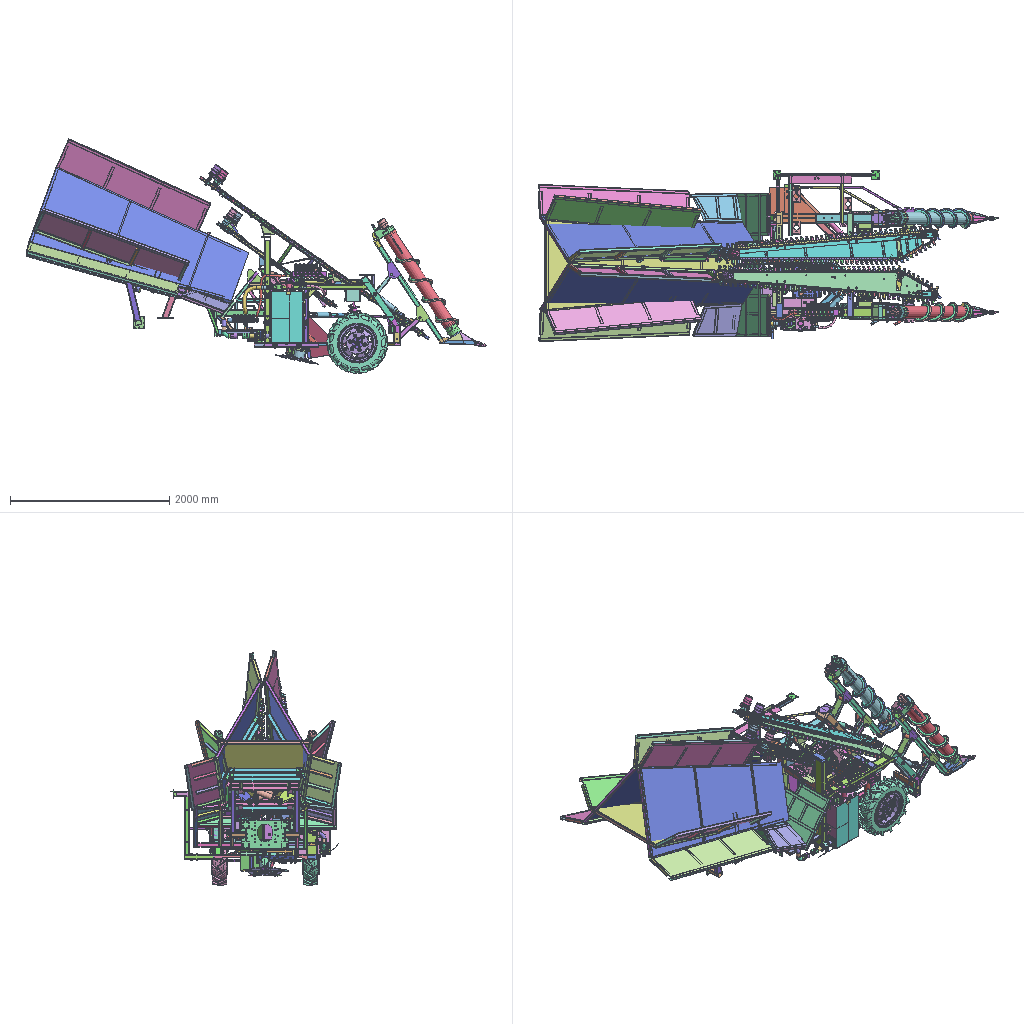Assembly | STEP file | 173 different items | 615 placed | box 5779 x 2151 x 2951 mm
Parts list (item | name | quantity | parent item | size | volume):
1 | 1 exported frame why_stp | x1 | in sugarcane cutter-windrower module--20251214 | 80 x 1320 x 1285 mm | 10409301 mm3
2 | floating channel bottom plate--2025.12.03 | x1 | in floating channel--20251204 | 466.015 x 268.5 x 616.159 mm | 643321 mm3
3 | floating channel right front section | x1 | in floating channel--20251204 | 394.503 x 166.964 x 591.584 mm | 406716 mm3
4 | floating channel left front section | x1 | in floating channel--20251204 | 372.026 x 168.494 x 590.246 mm | 526748 mm3
5 | floating channel side plate | x1 | in floating channel--20251204 | 471.639 x 3 x 716.945 mm | 405193 mm3
6 | floating channel side plate 02 | x1 | in floating channel--20251204 | 470.946 x 3 x 716.27 mm | 404515 mm3
7 | support fixing frame | x1 | in floating channel fixing frame_MODEL | 66.075 x 284.5 x 50.67 mm | 158932 mm3
8 | vertical fixing frame | x1 | in floating channel fixing frame_MODEL | 87.186 x 40 x 183.865 mm | 87563 mm3
9 | diagonal bracket | x1 | in floating channel fixing frame_MODEL | 71.941 x 40 x 203.909 mm | 85272 mm3
10 | SOLID | x1 | in floating channel fixing frame_MODEL | 384.531 x 40 x 366.951 mm | 215519 mm3
11 | front baffle frame--20251202 | x1 | in front baffle fixing frame--20251202 | 468.919 x 1805 x 743.614 mm | 3730425 mm3
12 | front baffle frame | x1 | in front baffle fixing frame--20251202 | 240.241 x 40 x 360.346 mm | 161857 mm3
13 | right body front baffle fixing piece 2 | x1 | in right body front baffle fixing piece_MODEL | 373.425 x 40 x 40 mm | 150546 mm3
14 | SOLID | x1 | in right body front baffle fixing piece_MODEL | 216.705 x 40 x 40 mm | 84594 mm3
15 | _right fixed inclined baffle (down) | x1 | in fixed channel_MODEL--20251202 | 632.37 x 530.078 x 557.546 mm | 2099918 mm3
16 | left fixed inclined baffle (down) | x1 | in fixed channel_MODEL--20251202 | 733.286 x 530.621 x 522.776 mm | 2414380 mm3
17 | fixed baffle panel | x1 | in fixed channel_MODEL--20251202 | 439.017 x 1805 x 559.044 mm | 1940108 mm3
18 | COMPOUND | x1 | in fixed channel_MODEL--20251202 | 271.977 x 175 x 432.84 mm | 323014 mm3
19 | HL4GZ-1.58.020 (cutter motor inlet/outlet flange) | x2 | in 砍蔗机构-2022.6.4(马达接头)_MODEL | 66.692 x 41 x 55.077 mm | 25659 mm3
20 | COMPOUND | x1 | in 砍蔗机构-2022.6.4(马达接头)_MODEL | 53.666 x 112 x 97.534 mm | 44207 mm3
21 | HL4GZ-1.313.024 (upper steering tie-rod weldment) | x2 | in 前悬架-2022.7.5_MODEL | 144.341 x 206.961 x 35 mm | 151003 mm3
22 | HL4GZ-1.313.025 (lower steering tie-rod weldment) | x2 | in 前悬架-2022.7.5_MODEL | 179.65 x 72.156 x 50 mm | 127271 mm3
23 | HL4GZ-1.313.026 (steering rod mounting seat) | x2 | in 前悬架-2022.7.5_MODEL | 120.001 x 187.5 x 196 mm | 489671 mm3
24 | HL4GZ-1.313.027 (front suspension bracket weldment) | x2 | in 前悬架-2022.7.5_MODEL | 200.001 x 340.001 x 190 mm | 984384 mm3
25 | HL4GZ-1.313.204 (front wheel mounting plate) | x2 | in 前悬架-2022.7.5_MODEL | 240 x 30.001 x 240 mm | 849969 mm3
26 | HL4GZ-1.313.201 (left steering shaft) | x1 | in 前悬架-2022.7.5_MODEL | 41 x 41 x 329 mm | 265914 mm3
27 | HL4GZ-1.313.211 (right steering shaft) | x1 | in 前悬架-2022.7.5_MODEL | 41 x 41 x 329 mm | 265914 mm3
28 | HL4GZ-1.313.206 (steering cylinder extension rod) | x2 | in 前悬架-2022.7.5_MODEL | 141.883 x 145.233 x 40 mm | 166510 mm3
29 | HL4GZ-1.313.202 (eye-ring mounting shaft) | x2 | in 前悬架-2022.7.5_MODEL | 40 x 40 x 125 mm | 55861 mm3
30 | COMPOUND | x1 | in 前悬架-2022.7.5_MODEL | - | 107297601 mm3
31 | HL4GZ-1.862.032 (cane-lifter upper swing arm weldment) | x2 | in HL4GZ-1.862.039 (right cane-lifter mechanism assembly)_MODEL_MODEL, HL4GZ-1.862.029 (left cane-lifter mechanism assembly)_MODEL_MODEL | 250.646 x 110 x 292.008 mm | 622631 mm3
32 | HL4GZ-1.862.293 (pillow block bearing) | x2 | in HL4GZ-1.862.039 (right cane-lifter mechanism assembly)_MODEL_MODEL, HL4GZ-1.862.029 (left cane-lifter mechanism assembly)_MODEL_MODEL | 126.394 x 135 x 95.577 mm | 264041 mm3
33 | HL4GZ-1.862.034 (flange rotating shaft) | x2 | in HL4GZ-1.862.039 (right cane-lifter mechanism assembly)_MODEL_MODEL, HL4GZ-1.862.029 (left cane-lifter mechanism assembly)_MODEL_MODEL | 113.701 x 120 x 117.252 mm | 202570 mm3
34 | HL4GZ-1.862.036MP (roller mounting base) | x2 | in HL4GZ-1.862.036 (cane-lifter frame weldment)_MODEL_MODEL | 238.392 x 170 x 206.608 mm | 617379 mm3
35 | COMPOUND | x2 | in HL4GZ-1.862.036 (cane-lifter frame weldment)_MODEL_MODEL | 1402 x 148 x 1427 mm | 4524661 mm3
36 | HL4GZ-1.862.035 (motor mounting bracket weldment) | x2 | in HL4GZ-1.862.039 (right cane-lifter mechanism assembly)_MODEL_MODEL, HL4GZ-1.862.029 (left cane-lifter mechanism assembly)_MODEL_MODEL | 281.601 x 178 x 183.899 mm | 825391 mm3
37 | HL4GZ-1.862.033 (cane-lifter lower swing arm weldment) | x2 | in HL4GZ-1.862.039 (right cane-lifter mechanism assembly)_MODEL_MODEL, HL4GZ-1.862.029 (left cane-lifter mechanism assembly)_MODEL_MODEL | 335.777 x 110 x 315.389 mm | 1087087 mm3
38 | HL4GZ-1.862.030 (right spiral roller shaft) | x1 | in HL4GZ-1.862.039 (right cane-lifter mechanism assembly)_MODEL_MODEL | 960.116 x 266 x 1342 mm | 5047297 mm3
39 | COMPOUND | x1 | in HL4GZ-1.862.039 (right cane-lifter mechanism assembly)_MODEL_MODEL | 1417 x 170.85 x 1608 mm | 1769847 mm3
40 | HL4GZ-1.862.040 (left spiral roller shaft) | x1 | in HL4GZ-1.862.029 (left cane-lifter mechanism assembly)_MODEL_MODEL | 960.116 x 266 x 1342 mm | 5047344 mm3
41 | COMPOUND | x1 | in HL4GZ-1.862.029 (left cane-lifter mechanism assembly)_MODEL_MODEL | 1441 x 170.85 x 1608 mm | 1889259 mm3
42 | HL4GZ-1.862.041 (cane-lifter mechanism mounting pin weldment) | x4 | in 扶蔗机构-2022.6.10_MODEL | 35 x 235 x 34.891 mm | 74372 mm3
43 | HL4GZ-1.58.105 (cane-lifter cylinder pin bushing) | x4 | in 扶蔗机构-2022.6.10_MODEL | 30 x 15 x 30 mm | 4505 mm3
44 | COMPOUND | x1 | in 扶蔗机构-2022.6.10_MODEL | 628.615 x 1399 x 812.176 mm | 2722476 mm3
45 | HL4GZ-1.30.205 (side guard rod 1) | x1 | in HL4GZ-1.30 sugarcane cutter-windrower frame 000.001-20251212_MODEL | 1018 x 292.057 x 25 mm | 224244 mm3
46 | HL4GZ-1.30.206 (side guard rod 2) | x1 | in HL4GZ-1.30 sugarcane cutter-windrower frame 000.001-20251212_MODEL | 1311 x 292.057 x 25 mm | 284985 mm3
47 | HL4GZ-1.30.214 (tip-cutting square tube guide sleeve) | x1 | in HL4GZ-1.30 sugarcane cutter-windrower frame 000.001-20251212_MODEL | - | -
48 | HL4GZ-1.30.033 (cylinder mounting seat 1 weldment) | x2 | in HL4GZ-1.30.050-1 (front frame weldment)--20251212_MODEL | 93 x 70 x 70 mm | 109193 mm3
49 | HL4GD-1.30.102 upper-deck ladder mounting plate--20251212 | x1 | in HL4GZ-1.30.050-1 (front frame weldment)--20251212_MODEL | 271 x 5 x 120 mm | 159189 mm3
50 | HL4GD-1.30.103XL cab extended floor plate | x1 | in HL4GD-1.30.103 cab extended floor plate weldment--20251214_MODEL | 790 x 120 x 3 mm | 282420 mm3
51 | 8902-M10 nut | x2 | in HL4GD-1.30.103 cab extended floor plate weldment--20251214_MODEL | 18.475 x 16 x 9.5 mm | 1522 mm3
52 | HL4GD-1.30.104 cab frame rear mounting plate--20251212 | x1 | in HL4GZ-1.30.050-1 (front frame weldment)--20251212_MODEL | 100 x 100 x 8 mm | 76249 mm3
53 | HL4GD-1.30.105 cab frame front mounting plate--20251212 | x1 | in HL4GZ-1.30.050-1 (front frame weldment)--20251212_MODEL | 190 x 130 x 8 mm | 190269 mm3
54 | HL4GD-1.30.106 cab frame side mounting plate--20251212 | x2 | in HL4GZ-1.30.050-1 (front frame weldment)--20251212_MODEL | 100 x 120 x 8 mm | 90459 mm3
55 | HL4GD-1.30.107 cab vibration-damping mounting bracket--20251212 | x3 | in HL4GZ-1.30.050-1 (front frame weldment)--20251212_MODEL | 100 x 160 x 45 mm | 90028 mm3
56 | HL4GD-1.30.108 base frame outer longitudinal beam--20251212 | x1 | in HL4GZ-1.30.050-1 (front frame weldment)--20251212_MODEL | 1250 x 40 x 60 mm | 1044524 mm3
57 | HL4GD-1.30.109 base frame front crossmember--20251212 | x1 | in HL4GZ-1.30.050-1 (front frame weldment)--20251212_MODEL | 40 x 580 x 60 mm | 484659 mm3
58 | HL4GD-1.30.110 base frame rear crossmember--20251212 | x1 | in HL4GZ-1.30.050-1 (front frame weldment)--20251212_MODEL | 40 x 450 x 60 mm | 376029 mm3
59 | HL4GD-1.30.111 base frame middle crossmember--20251212 | x1 | in HL4GZ-1.30.050-1 (front frame weldment)--20251212_MODEL | 40 x 740 x 60 mm | 618358 mm3
60 | HL4GD-1.30.112 base frame support longitudinal beam--20251212 | x2 | in HL4GZ-1.30.050-1 (front frame weldment)--20251212_MODEL | 414 x 60 x 40 mm | 345946 mm3
61 | HL4GD-1.30.113 base frame front support vertical beam--20251212 | x1 | in HL4GZ-1.30.050-1 (front frame weldment)--20251212_MODEL | 40 x 60 x 115 mm | 96096 mm3
62 | HL4GD-1.30.114_60×40封Plate--20251212 | x2 | in HL4GZ-1.30.050-1 (front frame weldment)--20251212_MODEL | 3 x 34 x 54 mm | 5508 mm3
63 | COMPOUND | x1 | in HL4GZ-1.30.050-1 (front frame weldment)--20251212_MODEL | 2329 x 1902 x 1425 mm | 39311271 mm3
64 | HL4GZ-1.581.017 (tank top mounting seat weldment) | x4 | in HL4GZ-1.581.015 (sugarcane cutter-windrower hydraulic tank weldment)_MODEL_MODEL | 60 x 40 x 60 mm | 38051 mm3
65 | HL4GZ-1.581.018 (tank bottom mounting seat weldment) | x2 | in HL4GZ-1.581.015 (sugarcane cutter-windrower hydraulic tank weldment)_MODEL_MODEL | 60 x 50 x 50 mm | 38451 mm3
66 | HL4GZ-1.581.020 (return pipe weldment) | x4 | in HL4GZ-1.581.015 (sugarcane cutter-windrower hydraulic tank weldment)_MODEL_MODEL | 35 x 35 x 570 mm | 62212 mm3
67 | HL4GZ-1.581.019 (radiator return pipe weldment) | x1 | in HL4GZ-1.581.015 (sugarcane cutter-windrower hydraulic tank weldment)_MODEL_MODEL | 47.343 x 41 x 592 mm | 83507 mm3
68 | COMPOUND | x1 | in HL4GZ-1.581.015 (sugarcane cutter-windrower hydraulic tank weldment)_MODEL_MODEL | 419 x 418 x 771 mm | 5464093 mm3
69 | HL4GZ-1.581.025 (variable pump outlet fitting weldment) | x1 | in sugarcane cutter-windrower hydraulic tank--20251213_MODEL | 60 x 97.67 x 134 mm | 92965 mm3
70 | HL4GZ-1.581.027 (variable pump inlet fitting) | x1 | in sugarcane cutter-windrower hydraulic tank--20251213_MODEL | 350.221 x 222 x 152.386 mm | 345083 mm3
71 | HL4GZ-1.581.029 (hydraulic tank outlet front flange) | x1 | in HL4GZ-1.581.028 (hydraulic tank outlet fitting)_MODEL_MODEL | 78 x 130 x 130 mm | 210630 mm3
72 | COMPOUND | x1 | in HL4GZ-1.581.028 (hydraulic tank outlet fitting)_MODEL_MODEL | 285 x 242.184 x 135.057 mm | 593050 mm3
73 | HL4GZ-1.581.031 (return filter fitting weldment) | x1 | in sugarcane cutter-windrower hydraulic tank--20251213_MODEL | 68 x 63.509 x 55 mm | 80125 mm3
74 | HL4GZ-1.581.102 (tank fixing seat) | x4 | in sugarcane cutter-windrower hydraulic tank--20251213_MODEL | 40 x 16 x 70 mm | 42647 mm3
75 | HL4GZ-1.581.103 (tank support seat) | x1 | in sugarcane cutter-windrower hydraulic tank--20251213_MODEL | 420 x 120 x 60 mm | 179158 mm3
76 | HL4GZ-1.581.104 (tank support seat rib) | x2 | in sugarcane cutter-windrower hydraulic tank--20251213_MODEL | 3 x 120 x 57 mm | 14370 mm3
77 | HL4GZ-1.581.108 (auxiliary valve bracket) | x1 | in sugarcane cutter-windrower hydraulic tank--20251213_MODEL | 502 x 90 x 60 mm | 213929 mm3
78 | HL4GZ-1.581.109 (auxiliary valve bracket fixing seat) | x2 | in sugarcane cutter-windrower hydraulic tank--20251213_MODEL | 70 x 90 x 35 mm | 44644 mm3
79 | HL4GZ-1.58.021 (variable pump inlet transition pipe) | x1 | in sugarcane cutter-windrower hydraulic tank--20251213_MODEL | 168.5 x 168.5 x 237 mm | 261107 mm3
80 | 3521-20_plug 20 | x1 | in sugarcane cutter-windrower hydraulic tank--20251213_MODEL | 27 x 31.177 x 19.002 mm | 7988 mm3
81 | 8903-ZTZD20 combined gasket | x1 | in sugarcane cutter-windrower hydraulic tank--20251213_MODEL | 28 x 2 x 28 mm | 603.186 mm3
82 | COMPOUND | x1 | in sugarcane cutter-windrower hydraulic tank--20251213_MODEL | - | -
83 | COMPOUND | x1 | in HL4GZ-1.30 sugarcane cutter-windrower frame 000.001-20251212_MODEL | 2217 x 1725 x 986 mm | 1142087 mm3
84 | HL4GZ-1.862.045 (tensioner wheel mounting frame) | x3 | in HL4GZ-1.862.043 (left cane-feed mechanism assembly)_MODEL, driven wheel mounting frame, right cane-feed mechanism 0-2022.7.21_MODEL--2025.12.03 | 265.962 x 95.725 x 221.775 mm | 259615 mm3
85 | HL4GZ-1.862.046 (motor mounting seat) | x1 | in HL4GZ-1.862.043 (left cane-feed mechanism assembly)_MODEL | 187.193 x 135 x 210.336 mm | 284411 mm3
86 | HL4GZ-1.862.047 (left cane-feed mechanism frame) | x1 | in HL4GZ-1.862.043 (left cane-feed mechanism assembly)_MODEL | 2465 x 363.176 x 1756 mm | 3798659 mm3
87 | left cane-feed mechanism single-link chain | x1 | in HL4GZ-1.862.043 (left cane-feed mechanism assembly)_MODEL | 2616 x 545.862 x 1858 mm | 812261 mm3
88 | COMPOUND | x1 | in HL4GZ-1.862.043 (left cane-feed mechanism assembly)_MODEL | - | 3878446 mm3
89 | HL4GZ-1.30.038 (left cane-feed rear mounting seat weldment) | x1 | in Left送蔗机构-2022.7.21_MODEL--2025.12.03 | 173.767 x 270.5 x 171.433 mm | 416002 mm3
90 | HL4GZ-1.30.036 (left cane-feed front mounting seat weldment) | x1 | in Left送蔗机构-2022.7.21_MODEL--2025.12.03 | 173.767 x 392 x 282.649 mm | 650486 mm3
91 | rectangular upper-left | x2 | in upper conveyor bracket upper left_MODEL, right cane-feed mechanism 0-2022.7.21_MODEL--2025.12.03 | 80 x 500 x 80 mm | 574998 mm3
92 | COMPOUND | x1 | in upper conveyor bracket upper left_MODEL | 178.718 x 70 x 180.179 mm | 279954 mm3
93 | COMPOUND | x1 | in Left送蔗机构-2022.7.21_MODEL--2025.12.03 | 1791 x 180.745 x 1321 mm | 266287 mm3
94 | right conveyor single-link chain | x1 | in right cane-feed mechanism 0-2022.7.21_MODEL--2025.12.03 | 2497 x 489.718 x 1775 mm | 773582 mm3
95 | upper conveyor mechanism bracket right | x2 | in right cane-feed mechanism 0-2022.7.21_MODEL--2025.12.03 | 173.767 x 70 x 171.433 mm | 203728 mm3
96 | COMPOUND | x1 | in right cane-feed mechanism 0-2022.7.21_MODEL--2025.12.03 | - | 4143226 mm3
97 | upper-lower conveyor link bracket left | x1 | in upper-lower conveyor added bracket--20251204 | 480.245 x 142.878 x 467.818 mm | 564874 mm3
98 | upper-lower conveyor link bracket right | x1 | in upper-lower conveyor added bracket--20251204 | 481.108 x 232.016 x 467.858 mm | 606550 mm3
99 | tensioning conveyor mechanism lower bracket left 00 | x1 | in lower clamping conveyor mechanism right 60--2025.12.03 | 172.614 x 70 x 128.419 mm | 151635 mm3
100 | new extension bracket | x1 | in lower clamping conveyor mechanism right 60--2025.12.03 | 100.038 x 307.108 x 85.627 mm | 239797 mm3
101 | rectangular upper-left upper why latest oblique change--2025.12.03 | x1 | in lower clamping conveyor mechanism right 60--2025.12.03 | 140.025 x 315.696 x 108.411 mm | 564954 mm3
102 | COMPOUND | x1 | in lower clamping conveyor mechanism right 60--2025.12.03 | - | -
103 | rectangular upper-left upper why--2025.12.03 | x1 | in lower clamping conveyor mechanism left-left-right revised--2025.12.03 | 140 x 1021 x 130.016 mm | 912623 mm3
104 | tensioning conveyor mechanism lower bracket right | x1 | in lower clamping conveyor mechanism left-left-right revised--2025.12.03 | 178.949 x 70 x 168.419 mm | 258890 mm3
105 | COMPOUND | x1 | in lower clamping conveyor mechanism left-left-right revised--2025.12.03 | - | -
106 | HL4GZ-1.862.054 (gearbox mounting bracket weldment) | x1 | in HL4GZ-1.862.055 cutter mechanism_MODEL | 60 x 410 x 365.753 mm | 811040 mm3
107 | HL4GZ-1.862.057 (lower swing arm weldment) | x2 | in HL4GZ-1.862.055 cutter mechanism_MODEL | 184.383 x 266 x 76.55 mm | 187249 mm3
108 | HL4GZ-1.862.059 (gearbox housing) | x1 | in HL4GZ-1.862.055 cutter mechanism_MODEL | 222.162 x 305 x 145.748 mm | 1290088 mm3
109 | HL4GZ-1.862.060 (cutter disc mounting flange weldment) | x1 | in HL4GZ-1.862.055 cutter mechanism_MODEL | 246.616 x 250 x 233.706 mm | 1291217 mm3
110 | HL4GZ-1.862.061 (gearbox cover) | x1 | in HL4GZ-1.862.055 cutter mechanism_MODEL | 359.103 x 512.5 x 182.227 mm | 2369356 mm3
111 | HL4GZ-1.862.096 (cutter mechanism mounting seat weldment) | x1 | in HL4GZ-1.862.055 cutter mechanism_MODEL | 76 x 405 x 373 mm | 1546147 mm3
112 | HL4GZ-1.862.631 (blade mounting disc) | x1 | in HL4GZ-1.862.055 cutter mechanism_MODEL | 442.246 x 450 x 103.342 mm | 1520256 mm3
113 | HL4GZ-1.862.632 (blade) | x1 | in HL4GZ-1.862.055 cutter mechanism_MODEL | 543.655 x 584.18 x 120.404 mm | 403993 mm3
114 | HL4GZ-1.862.566 (lock washer) | x1 | in HL4GZ-1.862.055 cutter mechanism_MODEL | 71.466 x 75.5 x 19.86 mm | 12429 mm3
115 | HL4GZ-1.862.557 (lock nut) | x1 | in HL4GZ-1.862.055 cutter mechanism_MODEL | 67.997 x 67.816 x 23.464 mm | 19464 mm3
116 | HL4GZ-1.862.552 (cutter mechanism large gear) | x1 | in HL4GZ-1.862.055 cutter mechanism_MODEL | 144.135 x 140.903 x 58.656 mm | 353451 mm3
117 | HL4GZ-1.862.558 (flat washer GB_T 95 45) | x1 | in HL4GZ-1.862.055 cutter mechanism_MODEL | 79.915 x 80 x 24.458 mm | 26917 mm3
118 | HL4GZ-1.862.553 (cutter mechanism oil seal) | x2 | in HL4GZ-1.862.055 cutter mechanism_MODEL | 94.817 x 95 x 29.347 mm | 14495 mm3
119 | HL4GZ-1.862.556 (flat key) 16×10×30 | x1 | in HL4GZ-1.862.055 cutter mechanism_MODEL | 20.191 x 9 x 30.204 mm | 3929 mm3
120 | HL4GZ-1.862.554 (cutter mechanism bushing) | x1 | in HL4GZ-1.862.055 cutter mechanism_MODEL | 64.619 x 65 x 18.405 mm | 4582 mm3
121 | HL4GZ-1.862.551 (cutter mechanism pinion shaft) | x1 | in HL4GZ-1.862.055 cutter mechanism_MODEL | 65.702 x 59.943 x 82.24 mm | 96553 mm3
122 | HL4GZ-1.862.561 (elastic retaining ring -68) | x1 | in HL4GZ-1.862.055 cutter mechanism_MODEL | 67.9 x 71 x 16.767 mm | 2158 mm3
123 | 8903-010050 (O-ring) | x1 | in HL4GZ-1.862.055 cutter mechanism_MODEL | 97.924 x 100 x 24.752 mm | 5860 mm3
124 | HL4GZ-1.61.011 (hydraulic motor) | x1 | in HL4GZ-1.862.055 cutter mechanism_MODEL | 157.77 x 120 x 292.652 mm | 1969898 mm3
125 | HL4GZ-1.862.062 (anti-wrap blade seat) | x1 | in HL4GZ-1.862.055 cutter mechanism_MODEL | 96.231 x 100 x 118.639 mm | 177743 mm3
126 | HL4GZ-1.862.576 (bolt short shaft) | x1 | in HL4GZ-1.862.055 cutter mechanism_MODEL | 30 x 87 x 24 mm | 25136 mm3
127 | HL4GZ-1.862.562 (swing arm long shaft) | x2 | in HL4GZ-1.862.055 cutter mechanism_MODEL | 40 x 444.5 x 32 mm | 282616 mm3
128 | HL4GZ-1.862.565 swing arm short shaft | x2 | in HL4GZ-1.862.055 cutter mechanism_MODEL | 40 x 345 x 40 mm | 217186 mm3
129 | 8903-XA820 dowel pin (φ8×20) | x2 | in HL4GZ-1.862.055 cutter mechanism_MODEL | 13.634 x 10 x 21.56 mm | 1562 mm3
130 | 8901-M1030B (bolt M10×30) | x4 | in HL4GZ-1.862.055 cutter mechanism_MODEL | 21.132 x 18.475 x 43.007 mm | 4152 mm3
131 | 8902-10T (spring washer φ10) | x19 | in HL4GZ-1.862.055 cutter mechanism_MODEL | 15.587 x 15.4 x 5.745 mm | 264.776 mm3
132 | 8901-M1235B bolt M12×35 | x10 | in HL4GZ-1.862.055 cutter mechanism_MODEL | 23.601 x 20.671 x 44.467 mm | 6039 mm3
133 | 8092-12P flat washer | x30 | in HL4GZ-1.862.055 cutter mechanism_MODEL | 23.995 x 24 x 7.435 mm | 773.126 mm3
134 | 8901-M1240B bolt M12×40 | x5 | in HL4GZ-1.862.055 cutter mechanism_MODEL | 24.641 x 20.671 x 49.357 mm | 6605 mm3
135 | 8902-14P flat washer | x54 | in HL4GZ-1.862.055 cutter mechanism_MODEL | 27.908 x 28 x 8.267 mm | 1068 mm3
136 | 8902-M14 nut | x35 | in HL4GZ-1.862.055 cutter mechanism_MODEL | 25.147 x 23.458 x 16.886 mm | 3434 mm3
137 | 8902-14T spring washer | x34 | in HL4GZ-1.862.055 cutter mechanism_MODEL | 21.681 x 21.4 x 7.971 mm | 705.987 mm3
138 | 8901-M1445B bolt | x21 | in HL4GZ-1.862.055 cutter mechanism_MODEL | 29.442 x 21 x 56.008 mm | 10250 mm3
139 | HL4GZ-1.862.555 rolling bearing 7011 AC | x2 | in HL4GZ-1.862.055 cutter mechanism_MODEL | - | -
140 | 8903-ZC6008-2RS bearing 6008-2Z | x3 | in HL4GZ-1.862.055 cutter mechanism_MODEL | 69.261 x 68 x 28.438 mm | 22880 mm3
141 | 8901-M1040B (bolt M10×40) | x14 | in HL4GZ-1.862.055 cutter mechanism_MODEL | 23.234 x 16 x 47.898 mm | 4545 mm3
142 | 8901-M1050B (bolt M12×50) | x2 | in HL4GZ-1.862.055 cutter mechanism_MODEL | 24.329 x 18.475 x 57.75 mm | 5337 mm3
143 | HL4GZ-1.862.102 flat washer | x5 | in HL4GZ-1.862.055 cutter mechanism_MODEL | 40 x 5 x 40 mm | 5400 mm3
144 | 8901-M14 (bolt M14×95) | x7 | in HL4GZ-1.862.055 cutter mechanism_MODEL | 103.8 x 24.249 x 21 mm | 17952 mm3
145 | HL4GZ-1.30.033 (cylinder mounting seat 1 weldment) | x1 | in HL4GZ-1.862.055 cutter mechanism_MODEL | 93 x 80 x 100 mm | 131918 mm3
146 | _model23 | x1 | in HL4GZ-1.862.055 cutter mechanism_MODEL | 243.487 x 34 x 300.682 mm | 68472 mm3
147 | COMPOUND | x1 | in HL4GZ-1.862.055 cutter mechanism_MODEL | 412.654 x 246 x 1047 mm | 1106345 mm3
148 | fixing plate--000.001--20240925 | x12 | in left front support seat weldment--000.001--20240925, right front support seat weldment--000.001--20240925, frame rear support seat weldment--000.001--20240925 | 12 x 120 x 180 mm | 243659 mm3
149 | front support crossmember--000.001--20240925 | x6 | in left front support seat weldment--000.001--20240925, right front support seat weldment--000.001--20240925 | 80 x 176.5 x 60 mm | 218087 mm3
150 | front support column--000.001--20240925 | x6 | in left front support seat weldment--000.001--20240925, right front support seat weldment--000.001--20240925 | 483.278 x 60 x 348.303 mm | 654919 mm3
151 | front support mounting plate--000.001--20240925 | x6 | in left front support seat weldment--000.001--20240925, right front support seat weldment--000.001--20240925 | 162.121 x 12 x 167.799 mm | 242152 mm3
152 | COMPOUND | x6 | in frame rear support seat weldment--000.001--20240925 | 331.222 x 118 x 196.486 mm | 662464 mm3
153 | HL7YG-5.59.024_抓具油缸(缸体)--000.002--20240512 | x6 | in HL7YG-5.59.024_抓具油缸(63-32-420-220)(用于车厢翻转)--000.002--20240928, HL7YG-5.59.024_抓具油缸(63-32-420-220)(用于副车架翻转)--000.002--20240928 | 412.5 x 93.981 x 106.22 mm | 802630 mm3
154 | HL7YG-5.59.024_抓具油缸(活塞杆)--000.002--20240512 | x6 | in HL7YG-5.59.024_抓具油缸(63-32-420-220)(用于车厢翻转)--000.002--20240928, HL7YG-5.59.024_抓具油缸(63-32-420-220)(用于副车架翻转)--000.002--20240928 | 404.5 x 63 x 77.2 mm | 476577 mm3
155 | body floor longitudinal beam--000.001--20240926 | x6 | in body--000.001--20240926, body--000.001--20251202 | 40 x 40 x 2554 mm | 1074782 mm3
156 | body floor crossmember--000.001--20240926 | x3 | in body--000.001--20240926, body--000.001--20251202 | 60 x 887 x 40 mm | 741194 mm3
157 | body floor crossmember 1--000.001--20240926 | x3 | in body--000.001--20240926, body--000.001--20251202 | 60 x 1025 x 40 mm | 853212 mm3
158 | body tilt cylinder mounting plate 1--000.001--20240928 | x3 | in body--000.001--20240926, body--000.001--20251202 | 10 x 253.506 x 70 mm | 119523 mm3
159 | body tilt cylinder mounting plate 2--000.001--20240928 | x3 | in body--000.001--20240926, body--000.001--20251202 | 10 x 248.257 x 70 mm | 117424 mm3
160 | subframe tilt hinge plate--000.001--20240928 | x24 | in body--000.001--20240926, subframe weldment--000.001--20240908, body--000.001--20251202 | 10 x 50 x 120 mm | 52409 mm3
161 | COMPOUND | x1 | in body--000.001--20240926 | 325.47 x 1761 x 2548 mm | 11145517 mm3
162 | subframe cylinder mounting plate--000.001--20240928 | x6 | in subframe weldment--000.001--20240908 | 10 x 180 x 225 mm | 214706 mm3
163 | frame inner longitudinal beam--000.001--20240926 | x12 | in subframe weldment--000.001--20240908, main frame--000.001--20240928 | 40 x 280 x 60 mm | 242373 mm3
164 | frame crossmember 1--000.001--20240926 | x12 | in subframe weldment--000.001--20240908, main frame--000.001--20240928 | 837 x 40 x 60 mm | 699413 mm3
165 | frame crossmember 2-000.001--20240926 | x12 | in subframe weldment--000.001--20240908, main frame--000.001--20240928 | 887 x 40 x 60 mm | 731037 mm3
166 | subframe cylinder mounting plate reinforcement--000.001--20240928 | x3 | in subframe weldment--000.001--20240908 | 10 x 70 x 550 mm | 341000 mm3
167 | frame inner longitudinal beam 2--000.001--20240926 | x12 | in subframe weldment--000.001--20240908, main frame--000.001--20240928 | 40 x 110 x 60 mm | 95218 mm3
168 | frame longitudinal beam--000.001--20240926 | x12 | in subframe weldment--000.001--20240908, main frame--000.001--20240928 | 40 x 550 x 60 mm | 476091 mm3
169 | subframe tilt cylinder mounting plate--000.001--20240928 | x6 | in subframe weldment--000.001--20240908 | 10 x 215 x 70 mm | 131121 mm3
170 | cylinder mounting plate reinforcement--000.001--20240928 | x3 | in main frame--000.001--20240928 | 10 x 100 x 160 mm | 123785 mm3
171 | cylinder mounting plate--000.001--20240927 | x6 | in main frame--000.001--20240928 | 10 x 180 x 265 mm | 256557 mm3
172 | mounting plate--000.001--20240925 | x12 | in main frame--000.001--20240928 | 12 x 180 x 180 mm | 373259 mm3
173 | COMPOUND | x2 | in body--000.001--20251202 | 325.47 x 1761 x 2643 mm | 11287286 mm3
Placements (level | parent | child | x y z in mm | rotation matrix by rows), first 180 of 676 lines:
1 | sugarcane cutter-windrower module--20251214 | 1 exported frame why_stp | 0.0 0.0 0.0 | 1 0 0 0 1 0 0 0 1
1 | sugarcane cutter-windrower module--20251214 | floating channel--20251204 | 0.0 0.0 0.0 | 1 0 0 0 1 0 0 0 1
2 | floating channel--20251204 | floating channel bottom plate--2025.12.03 | 0.0 0.0 0.0 | 1 0 0 0 1 0 0 0 1
2 | floating channel--20251204 | floating channel right front section | 0.0 0.0 0.0 | 1 0 0 0 1 0 0 0 1
2 | floating channel--20251204 | floating channel left front section | 0.0 0.0 0.0 | 1 0 0 0 1 0 0 0 1
2 | floating channel--20251204 | floating channel side plate | 0.0 0.0 0.0 | 1 0 0 0 1 0 0 0 1
2 | floating channel--20251204 | floating channel side plate 02 | 0.0 0.0 0.0 | 1 0 0 0 1 0 0 0 1
2 | floating channel--20251204 | floating channel fixing frame_MODEL | 0.0 0.0 0.0 | 1 0 0 0 1 0 0 0 1
3 | floating channel fixing frame_MODEL | support fixing frame | 0.0 0.0 0.0 | 1 0 0 0 1 0 0 0 1
3 | floating channel fixing frame_MODEL | vertical fixing frame | 0.0 0.0 0.0 | 1 0 0 0 1 0 0 0 1
3 | floating channel fixing frame_MODEL | diagonal bracket | 0.0 0.0 0.0 | 1 0 0 0 1 0 0 0 1
3 | floating channel fixing frame_MODEL | SOLID | 0.0 0.0 0.0 | 1 0 0 0 1 0 0 0 1
1 | sugarcane cutter-windrower module--20251214 | fixed channel_MODEL--20251202 | 0.0 0.0 0.0 | 1 0 0 0 1 0 0 0 1
2 | fixed channel_MODEL--20251202 | front baffle fixing frame--20251202 | -46.985 -0.0 17.101 | 1 0 0 0 1 0 0 0 1
3 | front baffle fixing frame--20251202 | front baffle frame--20251202 | 9.173 0.0 -2.884 | 1 0 0 0 1 0 0 0 1
3 | front baffle fixing frame--20251202 | front baffle frame | -0.8269 0.0 -2.884 | 1 0 0 0 1 0 0 0 1
3 | front baffle fixing frame--20251202 | right body front baffle fixing piece_MODEL | 0.0 0.0 0.0 | 1 0 0 0 1 0 0 0 1
4 | right body front baffle fixing piece_MODEL | right body front baffle fixing piece 2 | 10.0 0.0 0.0 | 1 0 0 0 1 0 0 0 1
4 | right body front baffle fixing piece_MODEL | SOLID | 0.0 0.0 0.0 | 1 0 0 0 1 0 0 0 1
2 | fixed channel_MODEL--20251202 | _right fixed inclined baffle (down) | 13.055 -18.818 24.671 | 0.997 -0.02253 0.07455 0.02242 0.9997 0.002217 -0.07458 -0.000538 0.9972
2 | fixed channel_MODEL--20251202 | left fixed inclined baffle (down) | 35.455 -18.297 56.087 | 0.997 -0.02253 0.07455 0.02242 0.9997 0.002217 -0.07458 -0.000538 0.9972
2 | fixed channel_MODEL--20251202 | fixed baffle panel | 10.0 0.0 0.0 | 1 0 0 0 1 0 0 0 1
2 | fixed channel_MODEL--20251202 | COMPOUND | 0.0 0.0 0.0 | 1 0 0 0 1 0 0 0 1
1 | sugarcane cutter-windrower module--20251214 | HL4GZ-1.30 sugarcane cutter-windrower frame 000.001-20251212_MODEL | 0.0 0.0 0.0 | 1 0 0 0 1 0 0 0 1
2 | HL4GZ-1.30 sugarcane cutter-windrower frame 000.001-20251212_MODEL | 砍蔗机构-2022.6.4(马达接头)_MODEL | 0.0 0.0 0.0 | 1 0 0 0 1 0 0 0 1
3 | 砍蔗机构-2022.6.4(马达接头)_MODEL | HL4GZ-1.58.020 (cutter motor inlet/outlet flange) | 0.0 0.0 0.0 | 1 0 0 0 1 0 0 0 1
3 | 砍蔗机构-2022.6.4(马达接头)_MODEL | HL4GZ-1.58.020 (cutter motor inlet/outlet flange) | 945.491 -189 -1778.21 | 0.5592 0 0.829 0 -1 0 0.829 0 -0.5592
3 | 砍蔗机构-2022.6.4(马达接头)_MODEL | COMPOUND | 0.0 0.0 0.0 | 1 0 0 0 1 0 0 0 1
2 | HL4GZ-1.30 sugarcane cutter-windrower frame 000.001-20251212_MODEL | 前悬架-2022.7.5_MODEL | 0.0 0.0 0.0 | 1 0 0 0 1 0 0 0 1
3 | 前悬架-2022.7.5_MODEL | HL4GZ-1.313.024 (upper steering tie-rod weldment) | 0.0 0.0 0.0 | 1 0 0 0 1 0 0 0 1
3 | 前悬架-2022.7.5_MODEL | HL4GZ-1.313.024 (upper steering tie-rod weldment) | 3603.922 2210.479 0.0 | -0.4533 0.8914 0 -0.8914 -0.4533 0 0 0 1
3 | 前悬架-2022.7.5_MODEL | HL4GZ-1.313.025 (lower steering tie-rod weldment) | 0.0 0.0 0.0 | 1 0 0 0 1 0 0 0 1
3 | 前悬架-2022.7.5_MODEL | HL4GZ-1.313.025 (lower steering tie-rod weldment) | 0.0047 0.001 -572 | 1 0 0 0 -1 0 0 0 -1
3 | 前悬架-2022.7.5_MODEL | HL4GZ-1.313.026 (steering rod mounting seat) | 0.0 0.0 0.0 | 1 0 0 0 1 0 0 0 1
3 | 前悬架-2022.7.5_MODEL | HL4GZ-1.313.026 (steering rod mounting seat) | 5340.003 0.001 0.0 | -1 0 0 0 -1 0 0 0 1
3 | 前悬架-2022.7.5_MODEL | HL4GZ-1.313.027 (front suspension bracket weldment) | 0.0 0.0 0.0 | 1 0 0 0 1 0 0 0 1
3 | 前悬架-2022.7.5_MODEL | HL4GZ-1.313.027 (front suspension bracket weldment) | 5260.003 0.0016 0.0 | -1 0 0 0 -1 0 0 0 1
3 | 前悬架-2022.7.5_MODEL | HL4GZ-1.313.204 (front wheel mounting plate) | 0.0 0.0 0.0 | 1 0 0 0 1 0 0 0 1
3 | 前悬架-2022.7.5_MODEL | HL4GZ-1.313.204 (front wheel mounting plate) | 5253.641 0.0016 -1178.682 | -0.9042 -1e-06 0.4272 -1e-06 -1 -3e-06 0.4272 -3e-06 0.9042
3 | 前悬架-2022.7.5_MODEL | HL4GZ-1.313.201 (left steering shaft) | 0.0 0.0 0.0 | 1 0 0 0 1 0 0 0 1
3 | 前悬架-2022.7.5_MODEL | HL4GZ-1.313.211 (right steering shaft) | 0.0 0.0 0.0 | 1 0 0 0 1 0 0 0 1
3 | 前悬架-2022.7.5_MODEL | HL4GZ-1.313.206 (steering cylinder extension rod) | 0.0 0.0 0.0 | 1 0 0 0 1 0 0 0 1
3 | 前悬架-2022.7.5_MODEL | HL4GZ-1.313.202 (eye-ring mounting shaft) | 0.0 0.0 0.0 | 1 0 0 0 1 0 0 0 1
3 | 前悬架-2022.7.5_MODEL | HL4GZ-1.313.202 (eye-ring mounting shaft) | -0.0023 -296.077 0.0 | 1 0 0 0 1 0 0 0 1
3 | 前悬架-2022.7.5_MODEL | HL4GZ-1.313.206 (steering cylinder extension rod) | 2803.227 2712.423 -0.0 | -0.03292 0.9995 0 -0.9995 -0.03292 0 0 0 1
3 | 前悬架-2022.7.5_MODEL | COMPOUND | 0.0 0.0 0.0 | 1 0 0 0 1 0 0 0 1
2 | HL4GZ-1.30 sugarcane cutter-windrower frame 000.001-20251212_MODEL | 扶蔗机构-2022.6.10_MODEL | 0.0 0.0 0.0 | 1 0 0 0 1 0 0 0 1
3 | 扶蔗机构-2022.6.10_MODEL | HL4GZ-1.862.039 (right cane-lifter mechanism assembly)_MODEL_MODEL | 0.0 0.0 0.0 | 1 0 0 0 1 0 0 0 1
4 | HL4GZ-1.862.039 (right cane-lifter mechanism assembly)_MODEL_MODEL | HL4GZ-1.862.032 (cane-lifter upper swing arm weldment) | 0.0 -1180.0 0.0 | 1 0 0 0 1 0 0 0 1
4 | HL4GZ-1.862.039 (right cane-lifter mechanism assembly)_MODEL_MODEL | HL4GZ-1.862.293 (pillow block bearing) | 0.0 0.0 0.0 | 1 0 0 0 1 0 0 0 1
4 | HL4GZ-1.862.039 (right cane-lifter mechanism assembly)_MODEL_MODEL | HL4GZ-1.862.034 (flange rotating shaft) | 0.0 0.0 0.0 | 1 0 0 0 1 0 0 0 1
4 | HL4GZ-1.862.039 (right cane-lifter mechanism assembly)_MODEL_MODEL | HL4GZ-1.862.036 (cane-lifter frame weldment)_MODEL_MODEL | 0.0 0.0 0.0 | 1 0 0 0 1 0 0 0 1
5 | HL4GZ-1.862.036 (cane-lifter frame weldment)_MODEL_MODEL | HL4GZ-1.862.036MP (roller mounting base) | 0.0 -1180.0 0.0 | 1 0 0 0 1 0 0 0 1
5 | HL4GZ-1.862.036 (cane-lifter frame weldment)_MODEL_MODEL | COMPOUND | 0.0 0.0 0.0 | 1 0 0 0 1 0 0 0 1
4 | HL4GZ-1.862.039 (right cane-lifter mechanism assembly)_MODEL_MODEL | HL4GZ-1.862.035 (motor mounting bracket weldment) | 0.0 -1180.0 0.0 | 1 0 0 0 1 0 0 0 1
4 | HL4GZ-1.862.039 (right cane-lifter mechanism assembly)_MODEL_MODEL | HL4GZ-1.862.033 (cane-lifter lower swing arm weldment) | 0.0 -1180.0 0.0 | 1 0 0 0 1 0 0 0 1
4 | HL4GZ-1.862.039 (right cane-lifter mechanism assembly)_MODEL_MODEL | HL4GZ-1.862.030 (right spiral roller shaft) | 0.0 0.0 0.0 | 1 0 0 0 1 0 0 0 1
4 | HL4GZ-1.862.039 (right cane-lifter mechanism assembly)_MODEL_MODEL | COMPOUND | 0.0 0.0 0.0 | 1 0 0 0 1 0 0 0 1
3 | 扶蔗机构-2022.6.10_MODEL | HL4GZ-1.862.029 (left cane-lifter mechanism assembly)_MODEL_MODEL | 0.0 0.0 0.0 | 1 0 0 0 1 0 0 0 1
4 | HL4GZ-1.862.029 (left cane-lifter mechanism assembly)_MODEL_MODEL | HL4GZ-1.862.034 (flange rotating shaft) | 0.0 1180.0 -0.0 | 1 0 0 0 1 0 0 0 1
4 | HL4GZ-1.862.029 (left cane-lifter mechanism assembly)_MODEL_MODEL | HL4GZ-1.862.040 (left spiral roller shaft) | 0.0 0.0 0.0 | 1 0 0 0 1 0 0 0 1
4 | HL4GZ-1.862.029 (left cane-lifter mechanism assembly)_MODEL_MODEL | HL4GZ-1.862.035 (motor mounting bracket weldment) | 0.0 0.0 0.0 | 1 0 0 0 1 0 0 0 1
4 | HL4GZ-1.862.029 (left cane-lifter mechanism assembly)_MODEL_MODEL | HL4GZ-1.862.032 (cane-lifter upper swing arm weldment) | 0.0 0.0 0.0 | 1 0 0 0 1 0 0 0 1
4 | HL4GZ-1.862.029 (left cane-lifter mechanism assembly)_MODEL_MODEL | HL4GZ-1.862.033 (cane-lifter lower swing arm weldment) | 0.0 0.0 0.0 | 1 0 0 0 1 0 0 0 1
4 | HL4GZ-1.862.029 (left cane-lifter mechanism assembly)_MODEL_MODEL | HL4GZ-1.862.036 (cane-lifter frame weldment)_MODEL_MODEL | 0.0 1180.0 -0.0 | 1 0 0 0 1 0 0 0 1
5 | HL4GZ-1.862.036 (cane-lifter frame weldment)_MODEL_MODEL | HL4GZ-1.862.036MP (roller mounting base) | 0.0 -1180.0 0.0 | 1 0 0 0 1 0 0 0 1
5 | HL4GZ-1.862.036 (cane-lifter frame weldment)_MODEL_MODEL | COMPOUND | 0.0 0.0 0.0 | 1 0 0 0 1 0 0 0 1
4 | HL4GZ-1.862.029 (left cane-lifter mechanism assembly)_MODEL_MODEL | HL4GZ-1.862.293 (pillow block bearing) | 0.0 1180.0 -0.0 | 1 0 0 0 1 0 0 0 1
4 | HL4GZ-1.862.029 (left cane-lifter mechanism assembly)_MODEL_MODEL | COMPOUND | 0.0 0.0 0.0 | 1 0 0 0 1 0 0 0 1
3 | 扶蔗机构-2022.6.10_MODEL | HL4GZ-1.862.041 (cane-lifter mechanism mounting pin weldment) | 0.0 0.0 0.0 | 1 0 0 0 1 0 0 0 1
3 | 扶蔗机构-2022.6.10_MODEL | HL4GZ-1.862.041 (cane-lifter mechanism mounting pin weldment) | -276.815 0.0 561.944 | 1 0 0 0 1 0 0 0 1
3 | 扶蔗机构-2022.6.10_MODEL | HL4GZ-1.862.041 (cane-lifter mechanism mounting pin weldment) | -276.815 -1180.0 561.944 | 1 0 0 0 1 0 0 0 1
3 | 扶蔗机构-2022.6.10_MODEL | HL4GZ-1.862.041 (cane-lifter mechanism mounting pin weldment) | 0.0 -1180.0 0.0 | 1 0 0 0 1 0 0 0 1
3 | 扶蔗机构-2022.6.10_MODEL | HL4GZ-1.58.105 (cane-lifter cylinder pin bushing) | 0.0 0.0 0.0 | 1 0 0 0 1 0 0 0 1
3 | 扶蔗机构-2022.6.10_MODEL | HL4GZ-1.58.105 (cane-lifter cylinder pin bushing) | 0.0 1180.0 -0.0 | 1 0 0 0 1 0 0 0 1
3 | 扶蔗机构-2022.6.10_MODEL | HL4GZ-1.58.105 (cane-lifter cylinder pin bushing) | -0.0001 -0.0 20.622 | 1 0 0 0 -1 0 0 0 -1
3 | 扶蔗机构-2022.6.10_MODEL | HL4GZ-1.58.105 (cane-lifter cylinder pin bushing) | -0.0001 -1180.0 20.622 | 1 0 0 0 -1 0 0 0 -1
3 | 扶蔗机构-2022.6.10_MODEL | COMPOUND | 0.0 0.0 0.0 | 1 0 0 0 1 0 0 0 1
2 | HL4GZ-1.30 sugarcane cutter-windrower frame 000.001-20251212_MODEL | HL4GZ-1.30.205 (side guard rod 1) | 0.0 0.0 0.0 | 1 0 0 0 1 0 0 0 1
2 | HL4GZ-1.30 sugarcane cutter-windrower frame 000.001-20251212_MODEL | HL4GZ-1.30.206 (side guard rod 2) | 0.0 0.0 0.0 | 1 0 0 0 1 0 0 0 1
2 | HL4GZ-1.30 sugarcane cutter-windrower frame 000.001-20251212_MODEL | HL4GZ-1.30.214 (tip-cutting square tube guide sleeve) | 0.0 0.0 -800.0 | 1 0 0 0 1 0 0 0 1
2 | HL4GZ-1.30 sugarcane cutter-windrower frame 000.001-20251212_MODEL | HL4GZ-1.30.050-1 (front frame weldment)--20251212_MODEL | 0.0 0.0 0.0 | 1 0 0 0 1 0 0 0 1
3 | HL4GZ-1.30.050-1 (front frame weldment)--20251212_MODEL | HL4GZ-1.30.033 (cylinder mounting seat 1 weldment) | 0.0 0.0 0.0 | 1 0 0 0 1 0 0 0 1
3 | HL4GZ-1.30.050-1 (front frame weldment)--20251212_MODEL | HL4GZ-1.30.033 (cylinder mounting seat 1 weldment) | 0.009 1180.009 0.0 | 1 0 0 0 1 0 0 0 1
3 | HL4GZ-1.30.050-1 (front frame weldment)--20251212_MODEL | HL4GD-1.30.102 upper-deck ladder mounting plate--20251212 | 0.0 0.0 0.0 | 1 0 0 0 1 0 0 0 1
3 | HL4GZ-1.30.050-1 (front frame weldment)--20251212_MODEL | HL4GD-1.30.103 cab extended floor plate weldment--20251214_MODEL | 0.0 0.0 0.0 | 1 0 0 0 1 0 0 0 1
4 | HL4GD-1.30.103 cab extended floor plate weldment--20251214_MODEL | HL4GD-1.30.103XL cab extended floor plate | 0.0 0.0 0.0 | 1 0 0 0 1 0 0 0 1
4 | HL4GD-1.30.103 cab extended floor plate weldment--20251214_MODEL | 8902-M10 nut | 2005.0 1090.0 465.0 | 1 0 0 0 1 0 0 0 1
4 | HL4GD-1.30.103 cab extended floor plate weldment--20251214_MODEL | 8902-M10 nut | 2045.0 1090.0 465.0 | 1 0 0 0 1 0 0 0 1
3 | HL4GZ-1.30.050-1 (front frame weldment)--20251212_MODEL | HL4GD-1.30.104 cab frame rear mounting plate--20251212 | 0.0 0.0 0.0 | 1 0 0 0 1 0 0 0 1
3 | HL4GZ-1.30.050-1 (front frame weldment)--20251212_MODEL | HL4GD-1.30.105 cab frame front mounting plate--20251212 | 0.0 0.0 0.0 | 1 0 0 0 1 0 0 0 1
3 | HL4GZ-1.30.050-1 (front frame weldment)--20251212_MODEL | HL4GD-1.30.106 cab frame side mounting plate--20251212 | 0.0 0.0 0.0 | 1 0 0 0 1 0 0 0 1
3 | HL4GZ-1.30.050-1 (front frame weldment)--20251212_MODEL | HL4GD-1.30.107 cab vibration-damping mounting bracket--20251212 | 0.0 0.0 0.0 | 1 0 0 0 1 0 0 0 1
3 | HL4GZ-1.30.050-1 (front frame weldment)--20251212_MODEL | HL4GD-1.30.108 base frame outer longitudinal beam--20251212 | 0.0 0.0 0.0 | 1 0 0 0 1 0 0 0 1
3 | HL4GZ-1.30.050-1 (front frame weldment)--20251212_MODEL | HL4GD-1.30.109 base frame front crossmember--20251212 | 0.0 0.0 0.0 | 1 0 0 0 1 0 0 0 1
3 | HL4GZ-1.30.050-1 (front frame weldment)--20251212_MODEL | HL4GD-1.30.110 base frame rear crossmember--20251212 | 0.0 0.0 0.0 | 1 0 0 0 1 0 0 0 1
3 | HL4GZ-1.30.050-1 (front frame weldment)--20251212_MODEL | HL4GD-1.30.111 base frame middle crossmember--20251212 | 0.0 0.0 0.0 | 1 0 0 0 1 0 0 0 1
3 | HL4GZ-1.30.050-1 (front frame weldment)--20251212_MODEL | HL4GD-1.30.112 base frame support longitudinal beam--20251212 | 0.0 0.0 0.0 | 1 0 0 0 1 0 0 0 1
3 | HL4GZ-1.30.050-1 (front frame weldment)--20251212_MODEL | HL4GD-1.30.113 base frame front support vertical beam--20251212 | 0.0 0.0 0.0 | 1 0 0 0 1 0 0 0 1
3 | HL4GZ-1.30.050-1 (front frame weldment)--20251212_MODEL | HL4GD-1.30.114_60×40封Plate--20251212 | 0.0 0.0 0.0 | 1 0 0 0 1 0 0 0 1
3 | HL4GZ-1.30.050-1 (front frame weldment)--20251212_MODEL | HL4GD-1.30.106 cab frame side mounting plate--20251212 | 4290.0 -0.0 938 | -1 0 0 0 1 0 0 0 -1
3 | HL4GZ-1.30.050-1 (front frame weldment)--20251212_MODEL | HL4GD-1.30.107 cab vibration-damping mounting bracket--20251212 | 0.0 399.0 0.0 | 1 0 0 0 1 0 0 0 1
3 | HL4GZ-1.30.050-1 (front frame weldment)--20251212_MODEL | HL4GD-1.30.107 cab vibration-damping mounting bracket--20251212 | 650.0 299.0 0.0 | 1 0 0 0 1 0 0 0 1
3 | HL4GZ-1.30.050-1 (front frame weldment)--20251212_MODEL | HL4GD-1.30.112 base frame support longitudinal beam--20251212 | 0.0 60.0 -0.0 | 1 0 0 0 1 0 0 0 1
3 | HL4GZ-1.30.050-1 (front frame weldment)--20251212_MODEL | HL4GD-1.30.114_60×40封Plate--20251212 | 1253.0 -0.0 0.0 | 1 0 0 0 1 0 0 0 1
3 | HL4GZ-1.30.050-1 (front frame weldment)--20251212_MODEL | COMPOUND | 0.0 0.0 0.0 | 1 0 0 0 1 0 0 0 1
2 | HL4GZ-1.30 sugarcane cutter-windrower frame 000.001-20251212_MODEL | sugarcane cutter-windrower hydraulic tank--20251213_MODEL | 0.0 0.0 0.0 | 1 0 0 0 1 0 0 0 1
3 | sugarcane cutter-windrower hydraulic tank--20251213_MODEL | HL4GZ-1.581.015 (sugarcane cutter-windrower hydraulic tank weldment)_MODEL_MODEL | 0.0 0.0 0.0 | 1 0 0 0 1 0 0 0 1
4 | HL4GZ-1.581.015 (sugarcane cutter-windrower hydraulic tank weldment)_MODEL_MODEL | HL4GZ-1.581.017 (tank top mounting seat weldment) | 3607.0 -10.0 190 | -1 0 0 0 1 0 0 0 -1
4 | HL4GZ-1.581.015 (sugarcane cutter-windrower hydraulic tank weldment)_MODEL_MODEL | HL4GZ-1.581.017 (tank top mounting seat weldment) | 3607.0 -10.0 -150 | -1 0 0 0 1 0 0 0 -1
4 | HL4GZ-1.581.015 (sugarcane cutter-windrower hydraulic tank weldment)_MODEL_MODEL | HL4GZ-1.581.017 (tank top mounting seat weldment) | -0.0 0.0 340.0 | 1 0 0 0 1 0 0 0 1
4 | HL4GZ-1.581.015 (sugarcane cutter-windrower hydraulic tank weldment)_MODEL_MODEL | HL4GZ-1.581.017 (tank top mounting seat weldment) | 0.0 0.0 0.0 | 1 0 0 0 1 0 0 0 1
4 | HL4GZ-1.581.015 (sugarcane cutter-windrower hydraulic tank weldment)_MODEL_MODEL | HL4GZ-1.581.018 (tank bottom mounting seat weldment) | 0.0 0.0 0.0 | 1 0 0 0 1 0 0 0 1
4 | HL4GZ-1.581.015 (sugarcane cutter-windrower hydraulic tank weldment)_MODEL_MODEL | HL4GZ-1.581.018 (tank bottom mounting seat weldment) | 300.0 -0.0 -0.0 | 1 0 0 0 1 0 0 0 1
4 | HL4GZ-1.581.015 (sugarcane cutter-windrower hydraulic tank weldment)_MODEL_MODEL | HL4GZ-1.581.020 (return pipe weldment) | 2665.0 1180.0 -0.0 | 0 1 0 -1 0 0 0 0 1
4 | HL4GZ-1.581.015 (sugarcane cutter-windrower hydraulic tank weldment)_MODEL_MODEL | HL4GZ-1.581.020 (return pipe weldment) | 0.0 0.0 0.0 | 1 0 0 0 1 0 0 0 1
4 | HL4GZ-1.581.015 (sugarcane cutter-windrower hydraulic tank weldment)_MODEL_MODEL | HL4GZ-1.581.020 (return pipe weldment) | 1265.0 -2435.0 -0.0 | 0 -1 0 1 0 0 0 0 1
4 | HL4GZ-1.581.015 (sugarcane cutter-windrower hydraulic tank weldment)_MODEL_MODEL | HL4GZ-1.581.020 (return pipe weldment) | 1175.0 -2435.0 -0.0 | 0 -1 0 1 0 0 0 0 1
4 | HL4GZ-1.581.015 (sugarcane cutter-windrower hydraulic tank weldment)_MODEL_MODEL | HL4GZ-1.581.019 (radiator return pipe weldment) | 0.0 0.0 0.0 | 1 0 0 0 1 0 0 0 1
4 | HL4GZ-1.581.015 (sugarcane cutter-windrower hydraulic tank weldment)_MODEL_MODEL | COMPOUND | 0.0 0.0 0.0 | 1 0 0 0 1 0 0 0 1
3 | sugarcane cutter-windrower hydraulic tank--20251213_MODEL | HL4GZ-1.581.025 (variable pump outlet fitting weldment) | 0.0 0.0 0.0 | 1 0 0 0 1 0 0 0 1
3 | sugarcane cutter-windrower hydraulic tank--20251213_MODEL | HL4GZ-1.581.027 (variable pump inlet fitting) | 0.0 0.0 0.0 | 1 0 0 0 1 0 0 0 1
3 | sugarcane cutter-windrower hydraulic tank--20251213_MODEL | HL4GZ-1.581.028 (hydraulic tank outlet fitting)_MODEL_MODEL | 0.0 0.0 0.0 | 1 0 0 0 1 0 0 0 1
4 | HL4GZ-1.581.028 (hydraulic tank outlet fitting)_MODEL_MODEL | HL4GZ-1.581.029 (hydraulic tank outlet front flange) | 0.0 0.0 0.0 | 1 0 0 0 1 0 0 0 1
4 | HL4GZ-1.581.028 (hydraulic tank outlet fitting)_MODEL_MODEL | COMPOUND | 0.0 0.0 0.0 | 1 0 0 0 1 0 0 0 1
3 | sugarcane cutter-windrower hydraulic tank--20251213_MODEL | HL4GZ-1.581.031 (return filter fitting weldment) | 0.0 0.0 0.0 | 1 0 0 0 1 0 0 0 1
3 | sugarcane cutter-windrower hydraulic tank--20251213_MODEL | HL4GZ-1.581.102 (tank fixing seat) | 0.0 0.0 0.0 | 1 0 0 0 1 0 0 0 1
3 | sugarcane cutter-windrower hydraulic tank--20251213_MODEL | HL4GZ-1.581.102 (tank fixing seat) | -0.0 0.0 340.0 | 1 0 0 0 1 0 0 0 1
3 | sugarcane cutter-windrower hydraulic tank--20251213_MODEL | HL4GZ-1.581.102 (tank fixing seat) | -477.0 -10.0 340.0 | 1 0 0 0 1 0 0 0 1
3 | sugarcane cutter-windrower hydraulic tank--20251213_MODEL | HL4GZ-1.581.102 (tank fixing seat) | -477.0 -10.0 0.0 | 1 0 0 0 1 0 0 0 1
3 | sugarcane cutter-windrower hydraulic tank--20251213_MODEL | HL4GZ-1.581.103 (tank support seat) | 0.0 0.0 0.0 | 1 0 0 0 1 0 0 0 1
3 | sugarcane cutter-windrower hydraulic tank--20251213_MODEL | HL4GZ-1.581.104 (tank support seat rib) | 0.0 0.0 0.0 | 1 0 0 0 1 0 0 0 1
3 | sugarcane cutter-windrower hydraulic tank--20251213_MODEL | HL4GZ-1.581.104 (tank support seat rib) | -117.0 0.0 0.0 | 1 0 0 0 1 0 0 0 1
3 | sugarcane cutter-windrower hydraulic tank--20251213_MODEL | HL4GZ-1.581.108 (auxiliary valve bracket) | 0.0 0.0 0.0 | 1 0 0 0 1 0 0 0 1
3 | sugarcane cutter-windrower hydraulic tank--20251213_MODEL | HL4GZ-1.581.109 (auxiliary valve bracket fixing seat) | 0.0 0.0 0.0 | 1 0 0 0 1 0 0 0 1
3 | sugarcane cutter-windrower hydraulic tank--20251213_MODEL | HL4GZ-1.581.109 (auxiliary valve bracket fixing seat) | -460.0 0.0 0.0 | 1 0 0 0 1 0 0 0 1
3 | sugarcane cutter-windrower hydraulic tank--20251213_MODEL | HL4GZ-1.58.021 (variable pump inlet transition pipe) | 0.0 0.0 0.0 | 1 0 0 0 1 0 0 0 1
3 | sugarcane cutter-windrower hydraulic tank--20251213_MODEL | 3521-20_plug 20 | 1800.0 -740.0 -336.0 | 1 0 0 0 1 0 0 0 1
3 | sugarcane cutter-windrower hydraulic tank--20251213_MODEL | 8903-ZTZD20 combined gasket | 1800.0 -740.0 -336.0 | 1 0 0 0 0 -1 0 1 0
3 | sugarcane cutter-windrower hydraulic tank--20251213_MODEL | COMPOUND | 0.0 0.0 0.0 | 1 0 0 0 1 0 0 0 1
2 | HL4GZ-1.30 sugarcane cutter-windrower frame 000.001-20251212_MODEL | COMPOUND | 0.0 0.0 0.0 | 1 0 0 0 1 0 0 0 1
1 | sugarcane cutter-windrower module--20251214 | upper-lower conveyor added bracket--20251204 | 0.0 0.0 0.0 | 1 0 0 0 1 0 0 0 1
2 | upper-lower conveyor added bracket--20251204 | Left送蔗机构-2022.7.21_MODEL--2025.12.03 | 0.0 0.0 0.0 | 1 0 0 0 1 0 0 0 1
3 | Left送蔗机构-2022.7.21_MODEL--2025.12.03 | HL4GZ-1.862.043 (left cane-feed mechanism assembly)_MODEL | 0.0 0.0 0.0 | 1 0 0 0 1 0 0 0 1
4 | HL4GZ-1.862.043 (left cane-feed mechanism assembly)_MODEL | HL4GZ-1.862.045 (tensioner wheel mounting frame) | -16.027 207.521 11.315 | 0.9984 0.05699 0.001148 -0.05699 0.9976 0.04023 0.001148 -0.04023 0.9992
4 | HL4GZ-1.862.043 (left cane-feed mechanism assembly)_MODEL | HL4GZ-1.862.046 (motor mounting seat) | -1307.086 0.0 922.782 | 1 0 0 0 1 0 0 0 1
4 | HL4GZ-1.862.043 (left cane-feed mechanism assembly)_MODEL | HL4GZ-1.862.047 (left cane-feed mechanism frame) | 0.0 0.0 0.0 | 1 0 0 0 1 0 0 0 1
4 | HL4GZ-1.862.043 (left cane-feed mechanism assembly)_MODEL | left cane-feed mechanism single-link chain | 4186.254 413.88 1550.75 | -0.9833 -0.1814 -0.01176 -0.1814 0.975 0.1281 -0.01176 0.1281 -0.9917
4 | HL4GZ-1.862.043 (left cane-feed mechanism assembly)_MODEL | COMPOUND | 0.0 0.0 0.0 | 1 0 0 0 1 0 0 0 1
3 | Left送蔗机构-2022.7.21_MODEL--2025.12.03 | HL4GZ-1.30.038 (left cane-feed rear mounting seat weldment) | 0.0 101.666 0.0 | 1 0 0 0 1 0 0 0 1
3 | Left送蔗机构-2022.7.21_MODEL--2025.12.03 | HL4GZ-1.30.036 (left cane-feed front mounting seat weldment) | 0.0 0.0 0.0 | 1 0 0 0 1 0 0 0 1
3 | Left送蔗机构-2022.7.21_MODEL--2025.12.03 | upper conveyor bracket upper left_MODEL | -890.317 23.463 628.55 | 1 0 0 0 1 0 0 0 1
4 | upper conveyor bracket upper left_MODEL | rectangular upper-left | 16.065 -9.163 6.903 | 1 0 0 0 1 0 0 0 1
4 | upper conveyor bracket upper left_MODEL | COMPOUND | 0.0 0.0 0.0 | 1 0 0 0 1 0 0 0 1
3 | Left送蔗机构-2022.7.21_MODEL--2025.12.03 | driven wheel mounting frame | 0.0 0.0 0.0 | 1 0 0 0 1 0 0 0 1
4 | driven wheel mounting frame | HL4GZ-1.862.045 (tensioner wheel mounting frame) | -16.027 207.521 11.315 | 0.9984 0.05699 0.001148 -0.05699 0.9976 0.04023 0.001148 -0.04023 0.9992
3 | Left送蔗机构-2022.7.21_MODEL--2025.12.03 | COMPOUND | 0.0 0.0 0.0 | 1 0 0 0 1 0 0 0 1
2 | upper-lower conveyor added bracket--20251204 | right cane-feed mechanism 0-2022.7.21_MODEL--2025.12.03 | 0.0 0.0 0.0 | 1 0 0 0 1 0 0 0 1
3 | right cane-feed mechanism 0-2022.7.21_MODEL--2025.12.03 | right conveyor single-link chain | -17.608 -194.338 12.431 | 0.9984 -0.05699 0.001148 0.05699 0.9976 -0.04023 0.001148 0.04023 0.9992
3 | right cane-feed mechanism 0-2022.7.21_MODEL--2025.12.03 | rectangular upper-left | 3984.04 -6.818 635.312 | -1 0 0 0 -1 0 0 0 1
3 | right cane-feed mechanism 0-2022.7.21_MODEL--2025.12.03 | upper conveyor mechanism bracket right | -889.998 74.667 628.325 | 1 0 0 0 1 0 0 0 1
3 | right cane-feed mechanism 0-2022.7.21_MODEL--2025.12.03 | upper conveyor mechanism bracket right | 0.0 0.0 0.0 | 1 0 0 0 1 0 0 0 1
3 | right cane-feed mechanism 0-2022.7.21_MODEL--2025.12.03 | HL4GZ-1.862.045 (tensioner wheel mounting frame) | -16.794 -98.057 11.245 | 0.984 0.178 0.01132 -0.178 0.976 0.1257 0.01132 -0.1257 0.992
3 | right cane-feed mechanism 0-2022.7.21_MODEL--2025.12.03 | COMPOUND | 0.0 0.0 0.0 | 1 0 0 0 1 0 0 0 1
2 | upper-lower conveyor added bracket--20251204 | upper-lower conveyor link bracket left | 0.0 0.0 0.0 | 1 0 0 0 1 0 0 0 1
2 | upper-lower conveyor added bracket--20251204 | upper-lower conveyor link bracket right | 0.0 0.0 0.0 | 1 0 0 0 1 0 0 0 1
2 | upper-lower conveyor added bracket--20251204 | left-right clamping device revised 002--2025.12.03 | 0.0 -10.0 0.0 | 1 0 0 0 1 0 0 0 1
3 | left-right clamping device revised 002--2025.12.03 | lower clamping conveyor mechanism right 60--2025.12.03 | 1148.484 -1662.893 -80.078 | 0.4388 -0.8776 0.193 0.8944 0.4472 0 -0.0863 0.1726 0.9812
4 | lower clamping conveyor mechanism right 60--2025.12.03 | tensioning conveyor mechanism lower bracket left 00 | 912.101 1795.196 -114.989 | 0.4388 0.8944 -0.0863 -0.8776 0.4472 0.1726 0.193 0 0.9812
4 | lower clamping conveyor mechanism right 60--2025.12.03 | new extension bracket | 985.407 1769.888 -143.06 | 0.4388 0.8944 -0.0863 -0.8776 0.4472 0.1726 0.193 0 0.9812
4 | lower clamping conveyor mechanism right 60--2025.12.03 | rectangular upper-left upper why latest oblique change--2025.12.03 | 540.012 2623.541 -87.82 | 0.4388 0.8944 -0.0863 -0.8776 0.4472 0.1726 0.193 0 0.9812
4 | lower clamping conveyor mechanism right 60--2025.12.03 | COMPOUND | 0.0 0.0 0.0 | 1 0 0 0 1 0 0 0 1
3 | left-right clamping device revised 002--2025.12.03 | lower clamping conveyor mechanism left-left-right revised--2025.12.03 | 1148.484 -1920.534 -80.078 | 0.4388 -0.8776 0.193 0.8944 0.4472 0 -0.0863 0.1726 0.9812
4 | lower clamping conveyor mechanism left-left-right revised--2025.12.03 | rectangular upper-left upper why--2025.12.03 | 3042.039 -1476.584 853.522 | -0.4388 -0.8944 -0.0863 0.8776 -0.4472 0.1726 -0.193 0 0.9812
4 | lower clamping conveyor mechanism left-left-right revised--2025.12.03 | tensioning conveyor mechanism lower bracket right | 951.699 1814.944 -115.01 | 0.4388 0.8944 -0.0863 -0.8776 0.4472 0.1726 0.193 0 0.9812
4 | lower clamping conveyor mechanism left-left-right revised--2025.12.03 | COMPOUND | 0.0 0.0 0.0 | 1 0 0 0 1 0 0 0 1
1 | sugarcane cutter-windrower module--20251214 | HL4GZ-1.862.055 cutter mechanism_MODEL | 0.0 0.0 0.0 | 1 0 0 0 1 0 0 0 1
2 | HL4GZ-1.862.055 cutter mechanism_MODEL | HL4GZ-1.862.054 (gearbox mounting bracket weldment) | 0.0 0.0 0.0 | 1 0 0 0 1 0 0 0 1
2 | HL4GZ-1.862.055 cutter mechanism_MODEL | HL4GZ-1.862.057 (lower swing arm weldment) | 0.0 0.0 0.0 | 1 0 0 0 1 0 0 0 1
2 | HL4GZ-1.862.055 cutter mechanism_MODEL | HL4GZ-1.862.059 (gearbox housing) | 0.0 0.0 0.0 | 1 0 0 0 1 0 0 0 1